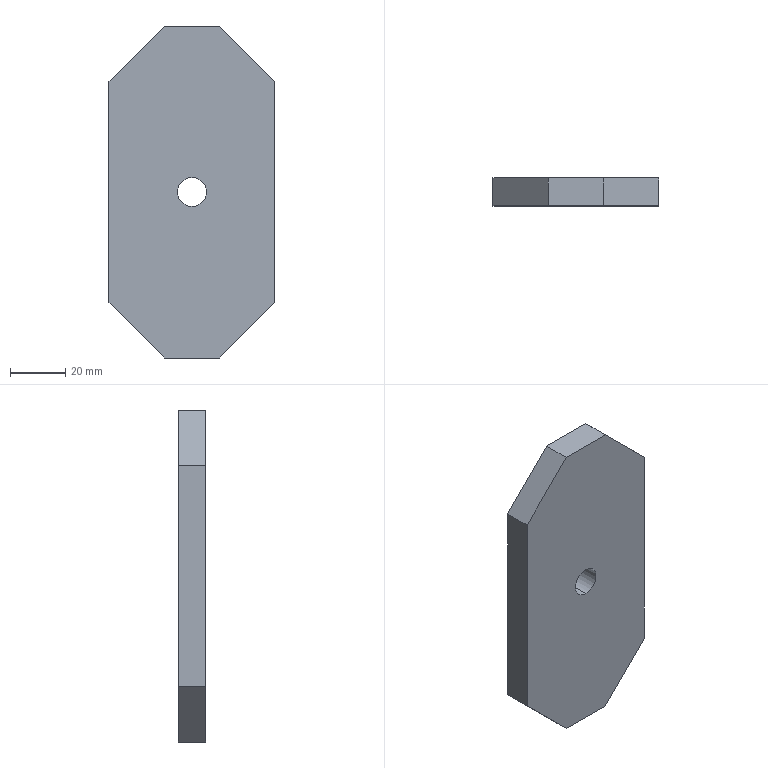Part | SolidWorks | features ICE 2, Chamfer 1, Extrusion 1 | 1 solid | 18 faces | box 60 x 10 x 120 mm | volume 62330 mm3 | plane 12 | cylinder 6 | commonest cylinder face diameters 16 x4 10.5 x2
STEP:
#1=CARTESIAN_POINT('',(0.,0.,-5.25));
#2=VERTEX_POINT('',#1);
#3=CARTESIAN_POINT('',(0.,0.,5.25));
#4=VERTEX_POINT('',#3);
#5=CARTESIAN_POINT('',(0.,0.,0.));
#6=DIRECTION('',(0.,1.,0.));
#7=DIRECTION('',(0.,0.,-1.));
#8=AXIS2_PLACEMENT_3D('',#5,#6,#7);
#9=CIRCLE('',#8,5.25);
#10=EDGE_CURVE('',#2,#4,#9,.T.);
#11=ORIENTED_EDGE('',*,*,#10,.F.);
#12=CARTESIAN_POINT('',(0.,10.,-5.25));
#13=VERTEX_POINT('',#12);
#14=CARTESIAN_POINT('',(0.,-0.001,-5.25));
#15=DIRECTION('',(0.,1.,0.));
#16=VECTOR('',#15,1000.);
#17=LINE('',#14,#16);
#18=EDGE_CURVE('',#2,#13,#17,.T.);
#19=ORIENTED_EDGE('',*,*,#18,.T.);
#20=CARTESIAN_POINT('',(0.,10.,5.25));
#21=VERTEX_POINT('',#20);
#22=CARTESIAN_POINT('',(0.,10.,0.));
#23=DIRECTION('',(0.,1.,0.));
#24=DIRECTION('',(0.,0.,1.));
#25=AXIS2_PLACEMENT_3D('',#22,#23,#24);
#26=CIRCLE('',#25,5.25);
#27=EDGE_CURVE('',#13,#21,#26,.T.);
#28=ORIENTED_EDGE('',*,*,#27,.T.);
#29=CARTESIAN_POINT('',(0.,-0.001,5.25));
#30=DIRECTION('',(0.,1.,0.));
#31=VECTOR('',#30,1000.);
#32=LINE('',#29,#31);
#33=EDGE_CURVE('',#4,#21,#32,.T.);
#34=ORIENTED_EDGE('',*,*,#33,.F.);
#35=EDGE_LOOP('',(#11,#19,#28,#34));
#36=FACE_OUTER_BOUND('',#35,.T.);
#37=CARTESIAN_POINT('',(0.,-0.001,0.));
#38=DIRECTION('',(0.,1.,0.));
#39=DIRECTION('',(0.,0.,1.));
#40=AXIS2_PLACEMENT_3D('',#37,#38,#39);
#41=CYLINDRICAL_SURFACE('',#40,5.25);
#42=ADVANCED_FACE('',(#36),#41,.F.);
#43=CARTESIAN_POINT('',(0.,8.,-54.));
#44=VERTEX_POINT('',#43);
#45=CARTESIAN_POINT('',(0.,8.,-38.));
#46=VERTEX_POINT('',#45);
#47=CARTESIAN_POINT('',(0.,8.,-46.));
#48=DIRECTION('',(0.,1.,0.));
#49=DIRECTION('',(0.,0.,1.));
#50=AXIS2_PLACEMENT_3D('',#47,#48,#49);
#51=CIRCLE('',#50,8.);
#52=EDGE_CURVE('',#44,#46,#51,.T.);
#53=ORIENTED_EDGE('',*,*,#52,.F.);
#54=CARTESIAN_POINT('',(0.,10.,-54.));
#55=VERTEX_POINT('',#54);
#56=CARTESIAN_POINT('',(0.,8.,-54.));
#57=DIRECTION('',(0.,1.,0.));
#58=VECTOR('',#57,1000.);
#59=LINE('',#56,#58);
#60=EDGE_CURVE('',#44,#55,#59,.T.);
#61=ORIENTED_EDGE('',*,*,#60,.T.);
#62=CARTESIAN_POINT('',(0.,10.,-38.));
#63=VERTEX_POINT('',#62);
#64=CARTESIAN_POINT('',(0.,10.,-46.));
#65=DIRECTION('',(0.,1.,0.));
#66=DIRECTION('',(0.,0.,1.));
#67=AXIS2_PLACEMENT_3D('',#64,#65,#66);
#68=CIRCLE('',#67,8.);
#69=EDGE_CURVE('',#55,#63,#68,.T.);
#70=ORIENTED_EDGE('',*,*,#69,.T.);
#71=CARTESIAN_POINT('',(0.,8.,-38.));
#72=DIRECTION('',(0.,1.,0.));
#73=VECTOR('',#72,1000.);
#74=LINE('',#71,#73);
#75=EDGE_CURVE('',#46,#63,#74,.T.);
#76=ORIENTED_EDGE('',*,*,#75,.F.);
#77=EDGE_LOOP('',(#53,#61,#70,#76));
#78=FACE_OUTER_BOUND('',#77,.T.);
#79=CARTESIAN_POINT('',(0.,8.,-46.));
#80=DIRECTION('',(0.,1.,0.));
#81=DIRECTION('',(0.,0.,1.));
#82=AXIS2_PLACEMENT_3D('',#79,#80,#81);
#83=CYLINDRICAL_SURFACE('',#82,8.);
#84=ADVANCED_FACE('',(#78),#83,.F.);
#85=CARTESIAN_POINT('',(0.,8.,38.));
#86=VERTEX_POINT('',#85);
#87=CARTESIAN_POINT('',(0.,8.,54.));
#88=VERTEX_POINT('',#87);
#89=CARTESIAN_POINT('',(0.,8.,46.));
#90=DIRECTION('',(0.,1.,0.));
#91=DIRECTION('',(0.,0.,1.));
#92=AXIS2_PLACEMENT_3D('',#89,#90,#91);
#93=CIRCLE('',#92,8.);
#94=EDGE_CURVE('',#86,#88,#93,.T.);
#95=ORIENTED_EDGE('',*,*,#94,.F.);
#96=CARTESIAN_POINT('',(0.,10.,38.));
#97=VERTEX_POINT('',#96);
#98=CARTESIAN_POINT('',(0.,8.,38.));
#99=DIRECTION('',(0.,1.,0.));
#100=VECTOR('',#99,1000.);
#101=LINE('',#98,#100);
#102=EDGE_CURVE('',#86,#97,#101,.T.);
#103=ORIENTED_EDGE('',*,*,#102,.T.);
#104=CARTESIAN_POINT('',(0.,10.,54.));
#105=VERTEX_POINT('',#104);
#106=CARTESIAN_POINT('',(0.,10.,46.));
#107=DIRECTION('',(0.,1.,0.));
#108=DIRECTION('',(0.,0.,1.));
#109=AXIS2_PLACEMENT_3D('',#106,#107,#108);
#110=CIRCLE('',#109,8.);
#111=EDGE_CURVE('',#97,#105,#110,.T.);
#112=ORIENTED_EDGE('',*,*,#111,.T.);
#113=CARTESIAN_POINT('',(0.,8.,54.));
#114=DIRECTION('',(0.,1.,0.));
#115=VECTOR('',#114,1000.);
#116=LINE('',#113,#115);
#117=EDGE_CURVE('',#88,#105,#116,.T.);
#118=ORIENTED_EDGE('',*,*,#117,.F.);
#119=EDGE_LOOP('',(#95,#103,#112,#118));
#120=FACE_OUTER_BOUND('',#119,.T.);
#121=CARTESIAN_POINT('',(0.,8.,46.));
#122=DIRECTION('',(0.,1.,0.));
#123=DIRECTION('',(0.,0.,1.));
#124=AXIS2_PLACEMENT_3D('',#121,#122,#123);
#125=CYLINDRICAL_SURFACE('',#124,8.);
#126=ADVANCED_FACE('',(#120),#125,.F.);
#127=CARTESIAN_POINT('',(30.,10.,40.));
#128=VERTEX_POINT('',#127);
#129=CARTESIAN_POINT('',(30.,10.,-40.));
#130=VERTEX_POINT('',#129);
#131=CARTESIAN_POINT('',(30.,10.,60.));
#132=DIRECTION('',(0.,0.,-1.));
#133=VECTOR('',#132,1000.);
#134=LINE('',#131,#133);
#135=EDGE_CURVE('',#128,#130,#134,.T.);
#136=ORIENTED_EDGE('',*,*,#135,.F.);
#137=CARTESIAN_POINT('',(30.,0.,40.));
#138=VERTEX_POINT('',#137);
#139=CARTESIAN_POINT('',(30.,10.,40.));
#140=DIRECTION('',(0.,-1.,0.));
#141=VECTOR('',#140,1000.);
#142=LINE('',#139,#141);
#143=EDGE_CURVE('',#128,#138,#142,.T.);
#144=ORIENTED_EDGE('',*,*,#143,.T.);
#145=CARTESIAN_POINT('',(30.,0.,-40.));
#146=VERTEX_POINT('',#145);
#147=CARTESIAN_POINT('',(30.,0.,60.));
#148=DIRECTION('',(0.,0.,-1.));
#149=VECTOR('',#148,1000.);
#150=LINE('',#147,#149);
#151=EDGE_CURVE('',#138,#146,#150,.T.);
#152=ORIENTED_EDGE('',*,*,#151,.T.);
#153=CARTESIAN_POINT('',(30.,10.,-40.));
#154=DIRECTION('',(0.,1.,0.));
#155=VECTOR('',#154,1000.);
#156=LINE('',#153,#155);
#157=EDGE_CURVE('',#146,#130,#156,.T.);
#158=ORIENTED_EDGE('',*,*,#157,.T.);
#159=EDGE_LOOP('',(#136,#144,#152,#158));
#160=FACE_OUTER_BOUND('',#159,.T.);
#161=CARTESIAN_POINT('',(30.,10.,60.));
#162=DIRECTION('',(-1.,0.,0.));
#163=DIRECTION('',(0.,0.,1.));
#164=AXIS2_PLACEMENT_3D('',#161,#162,#163);
#165=PLANE('',#164);
#166=ADVANCED_FACE('',(#160),#165,.F.);
#167=CARTESIAN_POINT('',(10.,10.,-60.));
#168=VERTEX_POINT('',#167);
#169=CARTESIAN_POINT('',(-10.,10.,-60.));
#170=VERTEX_POINT('',#169);
#171=CARTESIAN_POINT('',(-30.,10.,-60.));
#172=DIRECTION('',(-1.,0.,0.));
#173=VECTOR('',#172,1000.);
#174=LINE('',#171,#173);
#175=EDGE_CURVE('',#168,#170,#174,.T.);
#176=ORIENTED_EDGE('',*,*,#175,.F.);
#177=CARTESIAN_POINT('',(10.,0.,-60.));
#178=VERTEX_POINT('',#177);
#179=CARTESIAN_POINT('',(10.,10.,-60.));
#180=DIRECTION('',(0.,-1.,0.));
#181=VECTOR('',#180,1000.);
#182=LINE('',#179,#181);
#183=EDGE_CURVE('',#168,#178,#182,.T.);
#184=ORIENTED_EDGE('',*,*,#183,.T.);
#185=CARTESIAN_POINT('',(-10.,0.,-60.));
#186=VERTEX_POINT('',#185);
#187=CARTESIAN_POINT('',(-30.,0.,-60.));
#188=DIRECTION('',(-1.,0.,0.));
#189=VECTOR('',#188,1000.);
#190=LINE('',#187,#189);
#191=EDGE_CURVE('',#178,#186,#190,.T.);
#192=ORIENTED_EDGE('',*,*,#191,.T.);
#193=CARTESIAN_POINT('',(-10.,10.,-60.));
#194=DIRECTION('',(0.,1.,0.));
#195=VECTOR('',#194,1000.);
#196=LINE('',#193,#195);
#197=EDGE_CURVE('',#186,#170,#196,.T.);
#198=ORIENTED_EDGE('',*,*,#197,.T.);
#199=EDGE_LOOP('',(#176,#184,#192,#198));
#200=FACE_OUTER_BOUND('',#199,.T.);
#201=CARTESIAN_POINT('',(-30.,10.,-60.));
#202=DIRECTION('',(0.,0.,1.));
#203=DIRECTION('',(1.,0.,0.));
#204=AXIS2_PLACEMENT_3D('',#201,#202,#203);
#205=PLANE('',#204);
#206=ADVANCED_FACE('',(#200),#205,.F.);
#207=CARTESIAN_POINT('',(-30.,0.,-40.));
#208=VERTEX_POINT('',#207);
#209=CARTESIAN_POINT('',(-30.,0.,40.));
#210=VERTEX_POINT('',#209);
#211=CARTESIAN_POINT('',(-30.,0.,60.));
#212=DIRECTION('',(0.,0.,1.));
#213=VECTOR('',#212,1000.);
#214=LINE('',#211,#213);
#215=EDGE_CURVE('',#208,#210,#214,.T.);
#216=ORIENTED_EDGE('',*,*,#215,.T.);
#217=CARTESIAN_POINT('',(-30.,10.,40.));
#218=VERTEX_POINT('',#217);
#219=CARTESIAN_POINT('',(-30.,10.,40.));
#220=DIRECTION('',(0.,1.,0.));
#221=VECTOR('',#220,1000.);
#222=LINE('',#219,#221);
#223=EDGE_CURVE('',#210,#218,#222,.T.);
#224=ORIENTED_EDGE('',*,*,#223,.T.);
#225=CARTESIAN_POINT('',(-30.,10.,-40.));
#226=VERTEX_POINT('',#225);
#227=CARTESIAN_POINT('',(-30.,10.,60.));
#228=DIRECTION('',(0.,0.,1.));
#229=VECTOR('',#228,1000.);
#230=LINE('',#227,#229);
#231=EDGE_CURVE('',#226,#218,#230,.T.);
#232=ORIENTED_EDGE('',*,*,#231,.F.);
#233=CARTESIAN_POINT('',(-30.,10.,-40.));
#234=DIRECTION('',(0.,-1.,0.));
#235=VECTOR('',#234,1000.);
#236=LINE('',#233,#235);
#237=EDGE_CURVE('',#226,#208,#236,.T.);
#238=ORIENTED_EDGE('',*,*,#237,.T.);
#239=EDGE_LOOP('',(#216,#224,#232,#238));
#240=FACE_OUTER_BOUND('',#239,.T.);
#241=CARTESIAN_POINT('',(-30.,10.,60.));
#242=DIRECTION('',(1.,0.,0.));
#243=DIRECTION('',(0.,0.,-1.));
#244=AXIS2_PLACEMENT_3D('',#241,#242,#243);
#245=PLANE('',#244);
#246=ADVANCED_FACE('',(#240),#245,.F.);
#247=CARTESIAN_POINT('',(-10.,10.,60.));
#248=VERTEX_POINT('',#247);
#249=CARTESIAN_POINT('',(10.,10.,60.));
#250=VERTEX_POINT('',#249);
#251=CARTESIAN_POINT('',(-30.,10.,60.));
#252=DIRECTION('',(1.,0.,0.));
#253=VECTOR('',#252,1000.);
#254=LINE('',#251,#253);
#255=EDGE_CURVE('',#248,#250,#254,.T.);
#256=ORIENTED_EDGE('',*,*,#255,.F.);
#257=CARTESIAN_POINT('',(-10.,0.,60.));
#258=VERTEX_POINT('',#257);
#259=CARTESIAN_POINT('',(-10.,10.,60.));
#260=DIRECTION('',(0.,-1.,0.));
#261=VECTOR('',#260,1000.);
#262=LINE('',#259,#261);
#263=EDGE_CURVE('',#248,#258,#262,.T.);
#264=ORIENTED_EDGE('',*,*,#263,.T.);
#265=CARTESIAN_POINT('',(10.,0.,60.));
#266=VERTEX_POINT('',#265);
#267=CARTESIAN_POINT('',(-30.,0.,60.));
#268=DIRECTION('',(1.,0.,0.));
#269=VECTOR('',#268,1000.);
#270=LINE('',#267,#269);
#271=EDGE_CURVE('',#258,#266,#270,.T.);
#272=ORIENTED_EDGE('',*,*,#271,.T.);
#273=CARTESIAN_POINT('',(10.,10.,60.));
#274=DIRECTION('',(0.,1.,0.));
#275=VECTOR('',#274,1000.);
#276=LINE('',#273,#275);
#277=EDGE_CURVE('',#266,#250,#276,.T.);
#278=ORIENTED_EDGE('',*,*,#277,.T.);
#279=EDGE_LOOP('',(#256,#264,#272,#278));
#280=FACE_OUTER_BOUND('',#279,.T.);
#281=CARTESIAN_POINT('',(-30.,10.,60.));
#282=DIRECTION('',(0.,0.,-1.));
#283=DIRECTION('',(-1.,0.,0.));
#284=AXIS2_PLACEMENT_3D('',#281,#282,#283);
#285=PLANE('',#284);
#286=ADVANCED_FACE('',(#280),#285,.F.);
#287=CARTESIAN_POINT('',(0.,10.,0.));
#288=DIRECTION('',(0.,1.,0.));
#289=DIRECTION('',(0.,0.,1.));
#290=AXIS2_PLACEMENT_3D('',#287,#288,#289);
#291=CIRCLE('',#290,5.25);
#292=EDGE_CURVE('',#21,#13,#291,.T.);
#293=ORIENTED_EDGE('',*,*,#292,.F.);
#294=ORIENTED_EDGE('',*,*,#27,.F.);
#295=EDGE_LOOP('',(#293,#294));
#296=FACE_BOUND('',#295,.T.);
#297=CARTESIAN_POINT('',(0.,10.,-46.));
#298=DIRECTION('',(0.,1.,0.));
#299=DIRECTION('',(0.,0.,1.));
#300=AXIS2_PLACEMENT_3D('',#297,#298,#299);
#301=CIRCLE('',#300,8.);
#302=EDGE_CURVE('',#63,#55,#301,.T.);
#303=ORIENTED_EDGE('',*,*,#302,.F.);
#304=ORIENTED_EDGE('',*,*,#69,.F.);
#305=EDGE_LOOP('',(#303,#304));
#306=FACE_BOUND('',#305,.T.);
#307=CARTESIAN_POINT('',(0.,10.,46.));
#308=DIRECTION('',(0.,1.,0.));
#309=DIRECTION('',(0.,0.,1.));
#310=AXIS2_PLACEMENT_3D('',#307,#308,#309);
#311=CIRCLE('',#310,8.);
#312=EDGE_CURVE('',#105,#97,#311,.T.);
#313=ORIENTED_EDGE('',*,*,#312,.F.);
#314=ORIENTED_EDGE('',*,*,#111,.F.);
#315=EDGE_LOOP('',(#313,#314));
#316=FACE_BOUND('',#315,.T.);
#317=ORIENTED_EDGE('',*,*,#231,.T.);
#318=CARTESIAN_POINT('',(-10.,10.,60.));
#319=DIRECTION('',(0.7071,0.,0.7071));
#320=VECTOR('',#319,1000.);
#321=LINE('',#318,#320);
#322=EDGE_CURVE('',#218,#248,#321,.T.);
#323=ORIENTED_EDGE('',*,*,#322,.T.);
#324=ORIENTED_EDGE('',*,*,#255,.T.);
#325=CARTESIAN_POINT('',(30.,10.,40.));
#326=DIRECTION('',(0.7071,0.,-0.7071));
#327=VECTOR('',#326,1000.);
#328=LINE('',#325,#327);
#329=EDGE_CURVE('',#250,#128,#328,.T.);
#330=ORIENTED_EDGE('',*,*,#329,.T.);
#331=ORIENTED_EDGE('',*,*,#135,.T.);
#332=CARTESIAN_POINT('',(10.,10.,-60.));
#333=DIRECTION('',(-0.7071,0.,-0.7071));
#334=VECTOR('',#333,1000.);
#335=LINE('',#332,#334);
#336=EDGE_CURVE('',#130,#168,#335,.T.);
#337=ORIENTED_EDGE('',*,*,#336,.T.);
#338=ORIENTED_EDGE('',*,*,#175,.T.);
#339=CARTESIAN_POINT('',(-30.,10.,-40.));
#340=DIRECTION('',(-0.7071,0.,0.7071));
#341=VECTOR('',#340,1000.);
#342=LINE('',#339,#341);
#343=EDGE_CURVE('',#170,#226,#342,.T.);
#344=ORIENTED_EDGE('',*,*,#343,.T.);
#345=EDGE_LOOP('',(#317,#323,#324,#330,#331,#337,#338,#344));
#346=FACE_OUTER_BOUND('',#345,.T.);
#347=CARTESIAN_POINT('',(0.,10.,0.));
#348=DIRECTION('',(0.,-1.,0.));
#349=DIRECTION('',(0.,0.,-1.));
#350=AXIS2_PLACEMENT_3D('',#347,#348,#349);
#351=PLANE('',#350);
#352=ADVANCED_FACE('',(#296,#306,#316,#346),#351,.F.);
#353=CARTESIAN_POINT('',(0.,0.,0.));
#354=DIRECTION('',(0.,1.,0.));
#355=DIRECTION('',(0.,0.,-1.));
#356=AXIS2_PLACEMENT_3D('',#353,#354,#355);
#357=CIRCLE('',#356,5.25);
#358=EDGE_CURVE('',#4,#2,#357,.T.);
#359=ORIENTED_EDGE('',*,*,#358,.T.);
#360=ORIENTED_EDGE('',*,*,#10,.T.);
#361=EDGE_LOOP('',(#359,#360));
#362=FACE_BOUND('',#361,.T.);
#363=ORIENTED_EDGE('',*,*,#271,.F.);
#364=CARTESIAN_POINT('',(-35.,0.,35.));
#365=DIRECTION('',(-0.7071,0.,-0.7071));
#366=VECTOR('',#365,1000.);
#367=LINE('',#364,#366);
#368=EDGE_CURVE('',#258,#210,#367,.T.);
#369=ORIENTED_EDGE('',*,*,#368,.T.);
#370=ORIENTED_EDGE('',*,*,#215,.F.);
#371=CARTESIAN_POINT('',(-35.,0.,-35.));
#372=DIRECTION('',(0.7071,0.,-0.7071));
#373=VECTOR('',#372,1000.);
#374=LINE('',#371,#373);
#375=EDGE_CURVE('',#208,#186,#374,.T.);
#376=ORIENTED_EDGE('',*,*,#375,.T.);
#377=ORIENTED_EDGE('',*,*,#191,.F.);
#378=CARTESIAN_POINT('',(35.,0.,-35.));
#379=DIRECTION('',(0.7071,0.,0.7071));
#380=VECTOR('',#379,1000.);
#381=LINE('',#378,#380);
#382=EDGE_CURVE('',#178,#146,#381,.T.);
#383=ORIENTED_EDGE('',*,*,#382,.T.);
#384=ORIENTED_EDGE('',*,*,#151,.F.);
#385=CARTESIAN_POINT('',(35.,0.,35.));
#386=DIRECTION('',(-0.7071,0.,0.7071));
#387=VECTOR('',#386,1000.);
#388=LINE('',#385,#387);
#389=EDGE_CURVE('',#138,#266,#388,.T.);
#390=ORIENTED_EDGE('',*,*,#389,.T.);
#391=EDGE_LOOP('',(#363,#369,#370,#376,#377,#383,#384,#390));
#392=FACE_OUTER_BOUND('',#391,.T.);
#393=CARTESIAN_POINT('',(0.,0.,0.));
#394=DIRECTION('',(0.,-1.,0.));
#395=DIRECTION('',(0.,0.,-1.));
#396=AXIS2_PLACEMENT_3D('',#393,#394,#395);
#397=PLANE('',#396);
#398=ADVANCED_FACE('',(#362,#392),#397,.T.);
#399=ORIENTED_EDGE('',*,*,#102,.F.);
#400=CARTESIAN_POINT('',(0.,8.,46.));
#401=DIRECTION('',(0.,1.,0.));
#402=DIRECTION('',(0.,0.,1.));
#403=AXIS2_PLACEMENT_3D('',#400,#401,#402);
#404=CIRCLE('',#403,8.);
#405=EDGE_CURVE('',#88,#86,#404,.T.);
#406=ORIENTED_EDGE('',*,*,#405,.F.);
#407=ORIENTED_EDGE('',*,*,#117,.T.);
#408=ORIENTED_EDGE('',*,*,#312,.T.);
#409=EDGE_LOOP('',(#399,#406,#407,#408));
#410=FACE_OUTER_BOUND('',#409,.T.);
#411=CARTESIAN_POINT('',(0.,8.,46.));
#412=DIRECTION('',(0.,1.,0.));
#413=DIRECTION('',(0.,0.,1.));
#414=AXIS2_PLACEMENT_3D('',#411,#412,#413);
#415=CYLINDRICAL_SURFACE('',#414,8.);
#416=ADVANCED_FACE('',(#410),#415,.F.);
#417=ORIENTED_EDGE('',*,*,#405,.T.);
#418=ORIENTED_EDGE('',*,*,#94,.T.);
#419=EDGE_LOOP('',(#417,#418));
#420=FACE_OUTER_BOUND('',#419,.T.);
#421=CARTESIAN_POINT('',(0.,8.,46.));
#422=DIRECTION('',(0.,1.,0.));
#423=DIRECTION('',(0.,0.,1.));
#424=AXIS2_PLACEMENT_3D('',#421,#422,#423);
#425=PLANE('',#424);
#426=ADVANCED_FACE('',(#420),#425,.T.);
#427=ORIENTED_EDGE('',*,*,#60,.F.);
#428=CARTESIAN_POINT('',(0.,8.,-46.));
#429=DIRECTION('',(0.,1.,0.));
#430=DIRECTION('',(0.,0.,1.));
#431=AXIS2_PLACEMENT_3D('',#428,#429,#430);
#432=CIRCLE('',#431,8.);
#433=EDGE_CURVE('',#46,#44,#432,.T.);
#434=ORIENTED_EDGE('',*,*,#433,.F.);
#435=ORIENTED_EDGE('',*,*,#75,.T.);
#436=ORIENTED_EDGE('',*,*,#302,.T.);
#437=EDGE_LOOP('',(#427,#434,#435,#436));
#438=FACE_OUTER_BOUND('',#437,.T.);
#439=CARTESIAN_POINT('',(0.,8.,-46.));
#440=DIRECTION('',(0.,1.,0.));
#441=DIRECTION('',(0.,0.,1.));
#442=AXIS2_PLACEMENT_3D('',#439,#440,#441);
#443=CYLINDRICAL_SURFACE('',#442,8.);
#444=ADVANCED_FACE('',(#438),#443,.F.);
#445=ORIENTED_EDGE('',*,*,#433,.T.);
#446=ORIENTED_EDGE('',*,*,#52,.T.);
#447=EDGE_LOOP('',(#445,#446));
#448=FACE_OUTER_BOUND('',#447,.T.);
#449=CARTESIAN_POINT('',(0.,8.,-46.));
#450=DIRECTION('',(0.,1.,0.));
#451=DIRECTION('',(0.,0.,1.));
#452=AXIS2_PLACEMENT_3D('',#449,#450,#451);
#453=PLANE('',#452);
#454=ADVANCED_FACE('',(#448),#453,.T.);
#455=ORIENTED_EDGE('',*,*,#322,.F.);
#456=ORIENTED_EDGE('',*,*,#223,.F.);
#457=ORIENTED_EDGE('',*,*,#368,.F.);
#458=ORIENTED_EDGE('',*,*,#263,.F.);
#459=EDGE_LOOP('',(#455,#456,#457,#458));
#460=FACE_OUTER_BOUND('',#459,.T.);
#461=CARTESIAN_POINT('',(-10.,10.,60.));
#462=DIRECTION('',(0.7071,0.,-0.7071));
#463=DIRECTION('',(0.,-1.,0.));
#464=AXIS2_PLACEMENT_3D('',#461,#462,#463);
#465=PLANE('',#464);
#466=ADVANCED_FACE('',(#460),#465,.F.);
#467=ORIENTED_EDGE('',*,*,#329,.F.);
#468=ORIENTED_EDGE('',*,*,#277,.F.);
#469=ORIENTED_EDGE('',*,*,#389,.F.);
#470=ORIENTED_EDGE('',*,*,#143,.F.);
#471=EDGE_LOOP('',(#467,#468,#469,#470));
#472=FACE_OUTER_BOUND('',#471,.T.);
#473=CARTESIAN_POINT('',(30.,10.,40.));
#474=DIRECTION('',(-0.7071,0.,-0.7071));
#475=DIRECTION('',(0.,-1.,0.));
#476=AXIS2_PLACEMENT_3D('',#473,#474,#475);
#477=PLANE('',#476);
#478=ADVANCED_FACE('',(#472),#477,.F.);
#479=ORIENTED_EDGE('',*,*,#336,.F.);
#480=ORIENTED_EDGE('',*,*,#157,.F.);
#481=ORIENTED_EDGE('',*,*,#382,.F.);
#482=ORIENTED_EDGE('',*,*,#183,.F.);
#483=EDGE_LOOP('',(#479,#480,#481,#482));
#484=FACE_OUTER_BOUND('',#483,.T.);
#485=CARTESIAN_POINT('',(10.,10.,-60.));
#486=DIRECTION('',(-0.7071,0.,0.7071));
#487=DIRECTION('',(0.,-1.,0.));
#488=AXIS2_PLACEMENT_3D('',#485,#486,#487);
#489=PLANE('',#488);
#490=ADVANCED_FACE('',(#484),#489,.F.);
#491=ORIENTED_EDGE('',*,*,#343,.F.);
#492=ORIENTED_EDGE('',*,*,#197,.F.);
#493=ORIENTED_EDGE('',*,*,#375,.F.);
#494=ORIENTED_EDGE('',*,*,#237,.F.);
#495=EDGE_LOOP('',(#491,#492,#493,#494));
#496=FACE_OUTER_BOUND('',#495,.T.);
#497=CARTESIAN_POINT('',(-30.,10.,-40.));
#498=DIRECTION('',(0.7071,0.,0.7071));
#499=DIRECTION('',(0.,-1.,0.));
#500=AXIS2_PLACEMENT_3D('',#497,#498,#499);
#501=PLANE('',#500);
#502=ADVANCED_FACE('',(#496),#501,.F.);
#503=ORIENTED_EDGE('',*,*,#18,.F.);
#504=ORIENTED_EDGE('',*,*,#358,.F.);
#505=ORIENTED_EDGE('',*,*,#33,.T.);
#506=ORIENTED_EDGE('',*,*,#292,.T.);
#507=EDGE_LOOP('',(#503,#504,#505,#506));
#508=FACE_OUTER_BOUND('',#507,.T.);
#509=CARTESIAN_POINT('',(0.,-0.001,0.));
#510=DIRECTION('',(0.,1.,0.));
#511=DIRECTION('',(0.,0.,1.));
#512=AXIS2_PLACEMENT_3D('',#509,#510,#511);
#513=CYLINDRICAL_SURFACE('',#512,5.25);
#514=ADVANCED_FACE('',(#508),#513,.F.);
#515=CLOSED_SHELL('',(#42,#84,#126,#166,#206,#246,#286,#352,#398,#416,#426,#444,#454,#466,#478,#490,#502,#514));
#516=MANIFOLD_SOLID_BREP('',#515);
#517=CARTESIAN_POINT('',(0.,0.,0.));
#518=DIRECTION('',(0.,0.,1.));
#519=DIRECTION('',(1.,0.,0.));
#520=AXIS2_PLACEMENT_3D('',#517,#518,#519);
#521=(LENGTH_UNIT()NAMED_UNIT(*)SI_UNIT(.MILLI.,.METRE.));
#522=UNCERTAINTY_MEASURE_WITH_UNIT(LENGTH_MEASURE(0.00001),#521,'','');
#523=(NAMED_UNIT(*)PLANE_ANGLE_UNIT()SI_UNIT($,.RADIAN.));
#524=(NAMED_UNIT(*)SI_UNIT($,.STERADIAN.)SOLID_ANGLE_UNIT());
#525=(GEOMETRIC_REPRESENTATION_CONTEXT(3)GLOBAL_UNCERTAINTY_ASSIGNED_CONTEXT((#522))GLOBAL_UNIT_ASSIGNED_CONTEXT((#521,#523,#524))REPRESENTATION_CONTEXT('',''));
#526=ADVANCED_BREP_SHAPE_REPRESENTATION('',(#516,#520),#525);